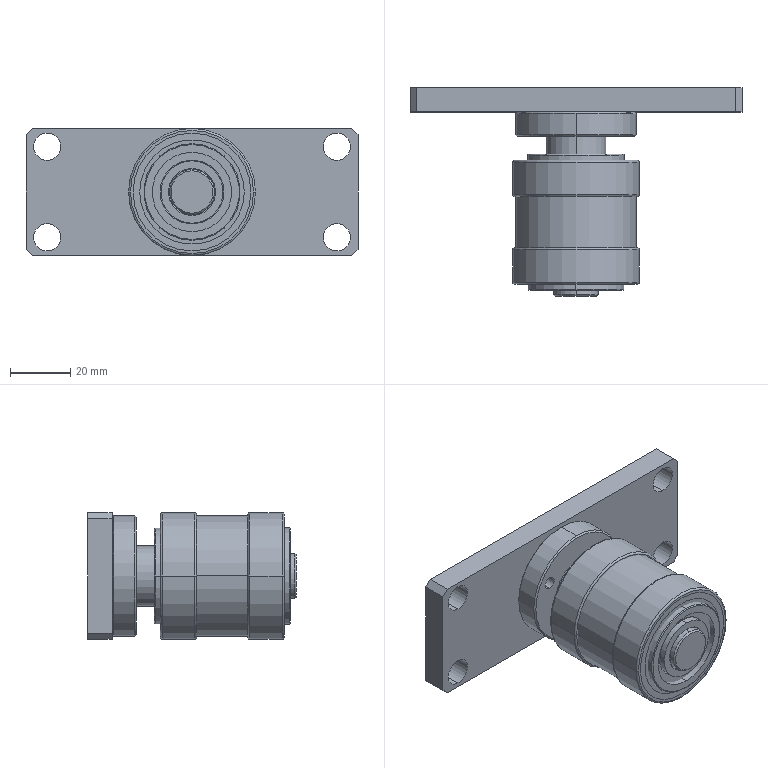Part | SolidWorks | 7 solids | 499 faces | box 110 x 69 x 42 mm | volume 113289 mm3 | torus 224 | sphere 128 | cylinder 92 | plane 39 | cone 16 | commonest cylinder face diameters 9 x8 15 x8 20.667 x8 26.333 x8 27.333 x8 34.667 x8